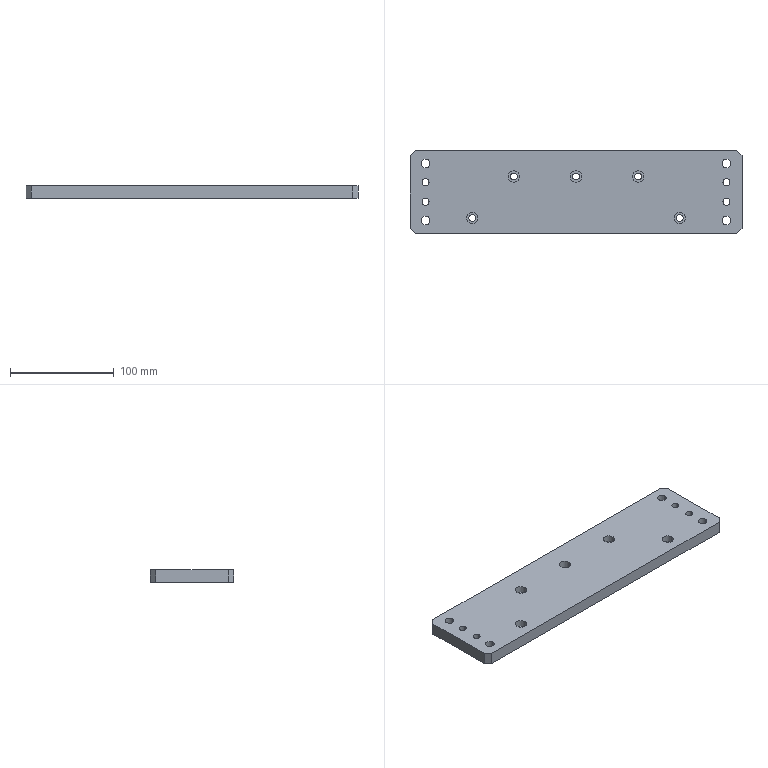Part | SolidWorks | features HoleWzd 3, Chamfer 1, Extrusion 1 | 1 solid | 51 faces | box 320 x 80 x 12 mm | volume 298012 mm3 | cylinder 36 | plane 15 | commonest cylinder face diameters 6.6 x10 11 x10 6.8 x8 8.5 x8